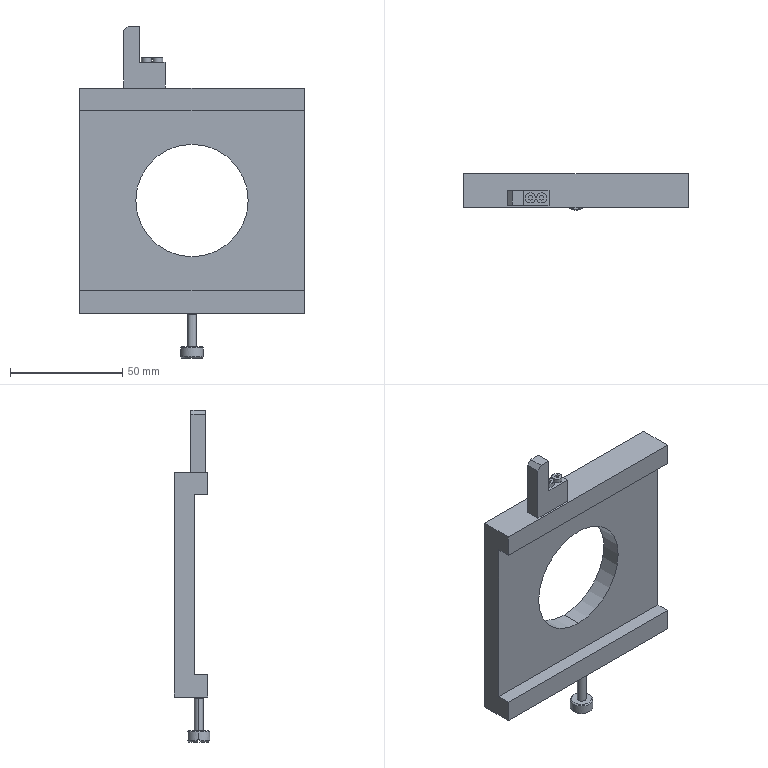Part | SolidWorks | features RevCut 12, ICE 7, Extrusion 1, Revolution 1 | 1 solid | 129 faces | box 100 x 16 x 147.6 mm | volume 86306 mm3 | cone 52 | plane 41 | cylinder 36 | commonest cylinder face diameters 3.242 x24 4.5 x4 2 x2 4 x2 10 x2 50 x2